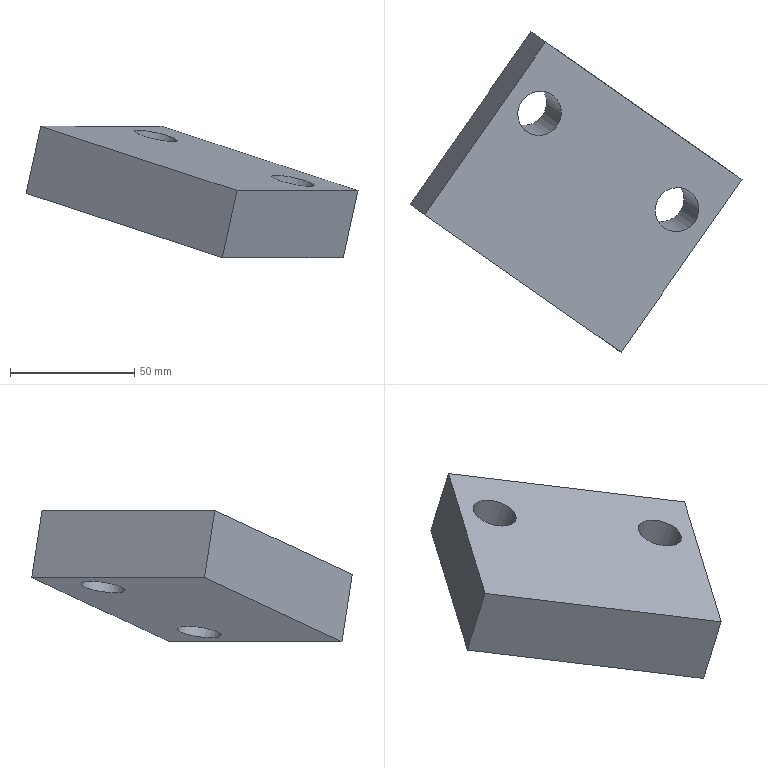Part | NX | features solid 2 | 1 solid | 8 faces | box 133.814 x 129.188 x 52.928 mm | volume 223750 mm3 | plane 6 | cylinder 2 | commonest cylinder face diameters 18 x2
STEP:
#1=CARTESIAN_POINT('',(-88.367,886.584,-40.822));
#2=VERTEX_POINT('',#1);
#3=CARTESIAN_POINT('',(-97.158,886.584,-38.892));
#4=DIRECTION('',(0.212,-0.1485,0.9659));
#5=DIRECTION('',(0.9767,0.,-0.2144));
#6=AXIS2_PLACEMENT_3D('',#3,#4,#5);
#7=CIRCLE('',#6,9.);
#8=EDGE_CURVE('',#2,#2,#7,.F.);
#9=ORIENTED_EDGE('',*,*,#8,.F.);
#10=EDGE_LOOP('',(#9));
#11=FACE_BOUND('',#10,.T.);
#12=CARTESIAN_POINT('',(-32.98,847.802,-58.939));
#13=VERTEX_POINT('',#12);
#14=CARTESIAN_POINT('',(-41.771,847.802,-57.009));
#15=DIRECTION('',(0.212,-0.1485,0.9659));
#16=DIRECTION('',(0.9767,0.,-0.2144));
#17=AXIS2_PLACEMENT_3D('',#14,#15,#16);
#18=CIRCLE('',#17,9.);
#19=EDGE_CURVE('',#13,#13,#18,.F.);
#20=ORIENTED_EDGE('',*,*,#19,.F.);
#21=EDGE_LOOP('',(#20));
#22=FACE_BOUND('',#21,.T.);
#23=CARTESIAN_POINT('',(-94.687,915.373,-35.01));
#24=VERTEX_POINT('',#23);
#25=CARTESIAN_POINT('',(-143.441,845.745,-35.01));
#26=VERTEX_POINT('',#25);
#27=CARTESIAN_POINT('',(-123.366,874.416,-35.01));
#28=DIRECTION('',(-0.5736,-0.8192,0.));
#29=VECTOR('',#28,1000.);
#30=LINE('',#27,#29);
#31=EDGE_CURVE('',#24,#26,#30,.T.);
#32=ORIENTED_EDGE('',*,*,#31,.F.);
#33=CARTESIAN_POINT('',(-15.563,859.97,-60.892));
#34=VERTEX_POINT('',#33);
#35=CARTESIAN_POINT('',(-73.938,900.845,-41.797));
#36=DIRECTION('',(-0.7912,0.554,0.2588));
#37=VECTOR('',#36,1000.);
#38=LINE('',#35,#37);
#39=EDGE_CURVE('',#24,#34,#38,.F.);
#40=ORIENTED_EDGE('',*,*,#39,.T.);
#41=CARTESIAN_POINT('',(-64.317,790.342,-60.892));
#42=VERTEX_POINT('',#41);
#43=CARTESIAN_POINT('',(-44.242,819.012,-60.892));
#44=DIRECTION('',(-0.5736,-0.8192,0.));
#45=VECTOR('',#44,1000.);
#46=LINE('',#43,#45);
#47=EDGE_CURVE('',#34,#42,#46,.T.);
#48=ORIENTED_EDGE('',*,*,#47,.T.);
#49=CARTESIAN_POINT('',(-122.692,831.217,-41.797));
#50=DIRECTION('',(-0.7912,0.554,0.2588));
#51=VECTOR('',#50,1000.);
#52=LINE('',#49,#51);
#53=EDGE_CURVE('',#26,#42,#52,.F.);
#54=ORIENTED_EDGE('',*,*,#53,.F.);
#55=EDGE_LOOP('',(#32,#40,#48,#54));
#56=FACE_BOUND('',#55,.T.);
#57=CARTESIAN_POINT('',(-102.617,859.887,-41.797));
#58=DIRECTION('',(-0.212,0.1485,-0.9659));
#59=DIRECTION('',(0.7912,-0.554,-0.2588));
#60=AXIS2_PLACEMENT_3D('',#57,#58,#59);
#61=PLANE('',#60);
#62=ADVANCED_FACE('',(#11,#22,#56),#61,.T.);
#63=CARTESIAN_POINT('',(-82.513,883.963,-13.522));
#64=VERTEX_POINT('',#63);
#65=CARTESIAN_POINT('',(-91.221,882.427,-11.846));
#66=DIRECTION('',(0.212,-0.1485,0.9659));
#67=DIRECTION('',(0.9676,0.1706,-0.1862));
#68=AXIS2_PLACEMENT_3D('',#65,#66,#67);
#69=CIRCLE('',#68,9.);
#70=EDGE_CURVE('',#64,#64,#69,.T.);
#71=ORIENTED_EDGE('',*,*,#70,.F.);
#72=EDGE_LOOP('',(#71));
#73=FACE_BOUND('',#72,.T.);
#74=CARTESIAN_POINT('',(-27.126,845.18,-31.639));
#75=VERTEX_POINT('',#74);
#76=CARTESIAN_POINT('',(-35.834,843.645,-29.963));
#77=DIRECTION('',(0.212,-0.1485,0.9659));
#78=DIRECTION('',(0.9676,0.1706,-0.1862));
#79=AXIS2_PLACEMENT_3D('',#76,#77,#78);
#80=CIRCLE('',#79,9.);
#81=EDGE_CURVE('',#75,#75,#80,.T.);
#82=ORIENTED_EDGE('',*,*,#81,.F.);
#83=EDGE_LOOP('',(#82));
#84=FACE_BOUND('',#83,.T.);
#85=CARTESIAN_POINT('',(-88.75,911.216,-7.964));
#86=VERTEX_POINT('',#85);
#87=CARTESIAN_POINT('',(-9.626,855.813,-33.846));
#88=VERTEX_POINT('',#87);
#89=CARTESIAN_POINT('',(-68.002,896.688,-14.751));
#90=DIRECTION('',(0.7912,-0.554,-0.2588));
#91=VECTOR('',#90,1000.);
#92=LINE('',#89,#91);
#93=EDGE_CURVE('',#86,#88,#92,.T.);
#94=ORIENTED_EDGE('',*,*,#93,.F.);
#95=CARTESIAN_POINT('',(-137.504,841.589,-7.964));
#96=VERTEX_POINT('',#95);
#97=CARTESIAN_POINT('',(-117.448,870.232,-7.964));
#98=DIRECTION('',(0.5736,0.8192,0.));
#99=VECTOR('',#98,1000.);
#100=LINE('',#97,#99);
#101=EDGE_CURVE('',#86,#96,#100,.F.);
#102=ORIENTED_EDGE('',*,*,#101,.T.);
#103=CARTESIAN_POINT('',(-58.38,786.185,-33.846));
#104=VERTEX_POINT('',#103);
#105=CARTESIAN_POINT('',(-116.756,827.06,-14.751));
#106=DIRECTION('',(0.7912,-0.554,-0.2588));
#107=VECTOR('',#106,1000.);
#108=LINE('',#105,#107);
#109=EDGE_CURVE('',#96,#104,#108,.T.);
#110=ORIENTED_EDGE('',*,*,#109,.T.);
#111=CARTESIAN_POINT('',(-38.324,814.829,-33.846));
#112=DIRECTION('',(0.5736,0.8192,0.));
#113=VECTOR('',#112,1000.);
#114=LINE('',#111,#113);
#115=EDGE_CURVE('',#88,#104,#114,.F.);
#116=ORIENTED_EDGE('',*,*,#115,.F.);
#117=EDGE_LOOP('',(#94,#102,#110,#116));
#118=FACE_BOUND('',#117,.T.);
#119=CARTESIAN_POINT('',(-96.681,855.73,-14.751));
#120=DIRECTION('',(-0.212,0.1485,-0.9659));
#121=DIRECTION('',(0.7912,-0.554,-0.2588));
#122=AXIS2_PLACEMENT_3D('',#119,#120,#121);
#123=PLANE('',#122);
#124=ADVANCED_FACE('',(#73,#84,#118),#123,.F.);
#125=CARTESIAN_POINT('',(-99.351,918.639,-56.26));
#126=DIRECTION('',(-0.212,0.1485,-0.9659));
#127=VECTOR('',#126,1000.);
#128=LINE('',#125,#127);
#129=EDGE_CURVE('',#24,#86,#128,.F.);
#130=ORIENTED_EDGE('',*,*,#129,.F.);
#131=ORIENTED_EDGE('',*,*,#31,.T.);
#132=CARTESIAN_POINT('',(-148.105,849.011,-56.26));
#133=DIRECTION('',(-0.212,0.1485,-0.9659));
#134=VECTOR('',#133,1000.);
#135=LINE('',#132,#134);
#136=EDGE_CURVE('',#26,#96,#135,.F.);
#137=ORIENTED_EDGE('',*,*,#136,.T.);
#138=ORIENTED_EDGE('',*,*,#101,.F.);
#139=EDGE_LOOP('',(#130,#131,#137,#138));
#140=FACE_BOUND('',#139,.T.);
#141=CARTESIAN_POINT('',(-117.11,869.996,-6.426));
#142=DIRECTION('',(-0.7912,0.554,0.2588));
#143=DIRECTION('',(0.5736,0.8192,0.));
#144=AXIS2_PLACEMENT_3D('',#141,#142,#143);
#145=PLANE('',#144);
#146=ADVANCED_FACE('',(#140),#145,.T.);
#147=ORIENTED_EDGE('',*,*,#109,.F.);
#148=ORIENTED_EDGE('',*,*,#136,.F.);
#149=ORIENTED_EDGE('',*,*,#53,.T.);
#150=CARTESIAN_POINT('',(-68.981,793.608,-82.142));
#151=DIRECTION('',(-0.212,0.1485,-0.9659));
#152=VECTOR('',#151,1000.);
#153=LINE('',#150,#152);
#154=EDGE_CURVE('',#42,#104,#153,.F.);
#155=ORIENTED_EDGE('',*,*,#154,.T.);
#156=EDGE_LOOP('',(#147,#148,#149,#155));
#157=FACE_BOUND('',#156,.T.);
#158=CARTESIAN_POINT('',(-127.356,834.483,-63.047));
#159=DIRECTION('',(0.5736,0.8192,0.));
#160=DIRECTION('',(0.8192,-0.5736,0.));
#161=AXIS2_PLACEMENT_3D('',#158,#159,#160);
#162=PLANE('',#161);
#163=ADVANCED_FACE('',(#157),#162,.F.);
#164=ORIENTED_EDGE('',*,*,#93,.T.);
#165=CARTESIAN_POINT('',(-20.227,863.236,-82.142));
#166=DIRECTION('',(-0.212,0.1485,-0.9659));
#167=VECTOR('',#166,1000.);
#168=LINE('',#165,#167);
#169=EDGE_CURVE('',#34,#88,#168,.F.);
#170=ORIENTED_EDGE('',*,*,#169,.F.);
#171=ORIENTED_EDGE('',*,*,#39,.F.);
#172=ORIENTED_EDGE('',*,*,#129,.T.);
#173=EDGE_LOOP('',(#164,#170,#171,#172));
#174=FACE_BOUND('',#173,.T.);
#175=CARTESIAN_POINT('',(-78.602,904.111,-63.047));
#176=DIRECTION('',(0.5736,0.8192,0.));
#177=DIRECTION('',(0.8192,-0.5736,0.));
#178=AXIS2_PLACEMENT_3D('',#175,#176,#177);
#179=PLANE('',#178);
#180=ADVANCED_FACE('',(#174),#179,.T.);
#181=ORIENTED_EDGE('',*,*,#169,.T.);
#182=ORIENTED_EDGE('',*,*,#115,.T.);
#183=ORIENTED_EDGE('',*,*,#154,.F.);
#184=ORIENTED_EDGE('',*,*,#47,.F.);
#185=EDGE_LOOP('',(#181,#182,#183,#184));
#186=FACE_BOUND('',#185,.T.);
#187=CARTESIAN_POINT('',(-37.986,814.593,-32.307));
#188=DIRECTION('',(-0.7912,0.554,0.2588));
#189=DIRECTION('',(0.5736,0.8192,0.));
#190=AXIS2_PLACEMENT_3D('',#187,#188,#189);
#191=PLANE('',#190);
#192=ADVANCED_FACE('',(#186),#191,.F.);
#193=ORIENTED_EDGE('',*,*,#19,.T.);
#194=EDGE_LOOP('',(#193));
#195=FACE_BOUND('',#194,.T.);
#196=ORIENTED_EDGE('',*,*,#81,.T.);
#197=EDGE_LOOP('',(#196));
#198=FACE_BOUND('',#197,.T.);
#199=CARTESIAN_POINT('',(-41.135,847.356,-54.112));
#200=DIRECTION('',(0.212,-0.1485,0.9659));
#201=DIRECTION('',(-0.9676,-0.1706,0.1862));
#202=AXIS2_PLACEMENT_3D('',#199,#200,#201);
#203=CYLINDRICAL_SURFACE('',#202,9.);
#204=ADVANCED_FACE('',(#195,#198),#203,.F.);
#205=ORIENTED_EDGE('',*,*,#8,.T.);
#206=EDGE_LOOP('',(#205));
#207=FACE_BOUND('',#206,.T.);
#208=ORIENTED_EDGE('',*,*,#70,.T.);
#209=EDGE_LOOP('',(#208));
#210=FACE_BOUND('',#209,.T.);
#211=CARTESIAN_POINT('',(-96.522,886.138,-35.994));
#212=DIRECTION('',(0.212,-0.1485,0.9659));
#213=DIRECTION('',(-0.9676,-0.1706,0.1862));
#214=AXIS2_PLACEMENT_3D('',#211,#212,#213);
#215=CYLINDRICAL_SURFACE('',#214,9.);
#216=ADVANCED_FACE('',(#207,#210),#215,.F.);
#217=CLOSED_SHELL('',(#62,#124,#146,#163,#180,#192,#204,#216));
#218=MANIFOLD_SOLID_BREP('',#217);
#219=(LENGTH_UNIT()NAMED_UNIT(*)SI_UNIT(.MILLI.,.METRE.));
#220=UNCERTAINTY_MEASURE_WITH_UNIT(LENGTH_MEASURE(0.00001),#219,'','');
#221=(NAMED_UNIT(*)PLANE_ANGLE_UNIT()SI_UNIT($,.RADIAN.));
#222=(NAMED_UNIT(*)SI_UNIT($,.STERADIAN.)SOLID_ANGLE_UNIT());
#223=(GEOMETRIC_REPRESENTATION_CONTEXT(3)GLOBAL_UNCERTAINTY_ASSIGNED_CONTEXT((#220))GLOBAL_UNIT_ASSIGNED_CONTEXT((#219,#221,#222))REPRESENTATION_CONTEXT('',''));
#224=ADVANCED_BREP_SHAPE_REPRESENTATION('',(#218),#223);